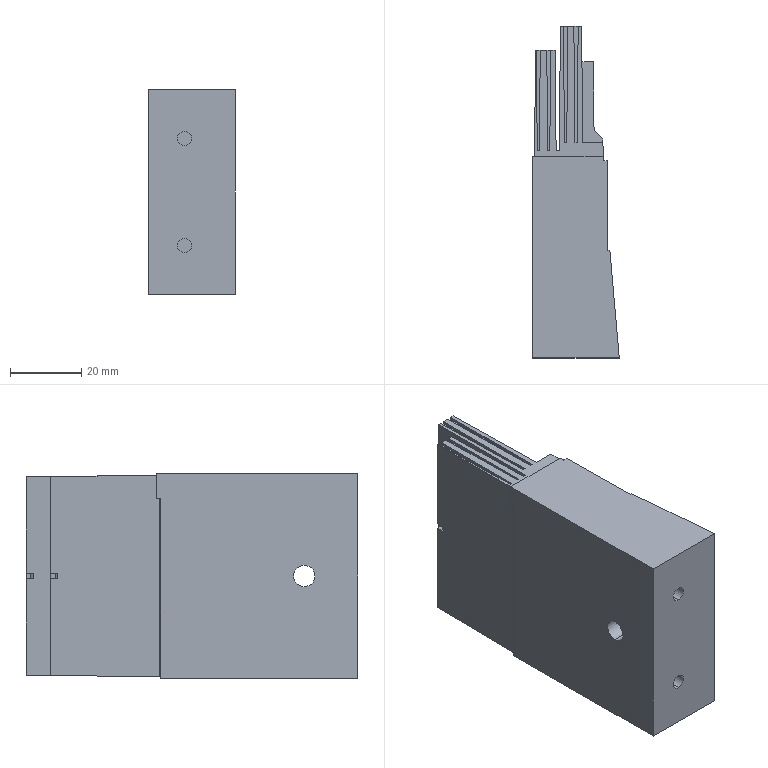Part | STEP file | 1 solid | 103 faces | box 24.206 x 92.813 x 57.276 mm | volume 94075 mm3 | plane 91 | cylinder 12 | commonest cylinder face diameters 1.005 x4 4 x4 6 x2 10 x2